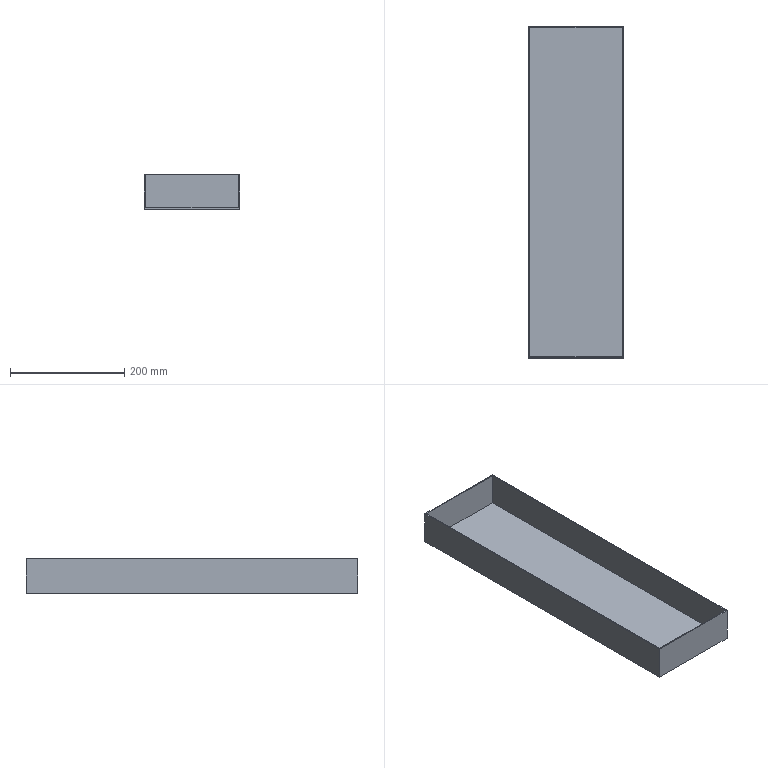Part | NX | features solid 2 | 1 solid | 11 faces | box 167 x 582.059 x 60 mm | volume 367262 mm3 | plane 9 | spline 2
STEP:
#1=CARTESIAN_POINT('',(-360.,302.059,-255.));
#2=VERTEX_POINT('',#1);
#3=CARTESIAN_POINT('',(-360.,-280.,-255.));
#4=VERTEX_POINT('',#3);
#5=CARTESIAN_POINT('',(-360.,-440.,-255.));
#6=DIRECTION('',(0.,1.,0.));
#7=VECTOR('',#6,1000.);
#8=LINE('',#5,#7);
#9=EDGE_CURVE('',#2,#4,#8,.F.);
#10=ORIENTED_EDGE('',*,*,#9,.T.);
#11=CARTESIAN_POINT('',(-360.,-280.,-315.));
#12=VERTEX_POINT('',#11);
#13=CARTESIAN_POINT('',(-360.,-280.,-315.));
#14=DIRECTION('',(0.,0.,1.));
#15=VECTOR('',#14,1000.);
#16=LINE('',#13,#15);
#17=EDGE_CURVE('',#12,#4,#16,.T.);
#18=ORIENTED_EDGE('',*,*,#17,.F.);
#19=CARTESIAN_POINT('',(-360.,302.059,-315.));
#20=VERTEX_POINT('',#19);
#21=CARTESIAN_POINT('',(-360.,-440.,-315.));
#22=DIRECTION('',(0.,1.,0.));
#23=VECTOR('',#22,1000.);
#24=LINE('',#21,#23);
#25=EDGE_CURVE('',#20,#12,#24,.F.);
#26=ORIENTED_EDGE('',*,*,#25,.F.);
#27=CARTESIAN_POINT('',(-360.,302.059,-285.));
#28=DIRECTION('',(0.,0.,1.));
#29=VECTOR('',#28,1000.);
#30=LINE('',#27,#29);
#31=EDGE_CURVE('',#20,#2,#30,.T.);
#32=ORIENTED_EDGE('',*,*,#31,.T.);
#33=EDGE_LOOP('',(#10,#18,#26,#32));
#34=FACE_BOUND('',#33,.T.);
#35=CARTESIAN_POINT('',(-360.,-440.,-315.));
#36=DIRECTION('',(-1.,0.,0.));
#37=DIRECTION('',(0.,0.,1.));
#38=AXIS2_PLACEMENT_3D('',#35,#36,#37);
#39=PLANE('',#38);
#40=ADVANCED_FACE('',(#34),#39,.F.);
#41=CARTESIAN_POINT('',(-527.,-280.,-255.));
#42=VERTEX_POINT('',#41);
#43=CARTESIAN_POINT('',(-780.,-280.,-255.));
#44=DIRECTION('',(-1.,0.,0.));
#45=VECTOR('',#44,1000.);
#46=LINE('',#43,#45);
#47=EDGE_CURVE('',#42,#4,#46,.F.);
#48=ORIENTED_EDGE('',*,*,#47,.F.);
#49=CARTESIAN_POINT('',(-527.,-280.,-315.));
#50=VERTEX_POINT('',#49);
#51=CARTESIAN_POINT('',(-527.,-280.,-315.));
#52=DIRECTION('',(0.,0.,1.));
#53=VECTOR('',#52,1000.);
#54=LINE('',#51,#53);
#55=EDGE_CURVE('',#50,#42,#54,.T.);
#56=ORIENTED_EDGE('',*,*,#55,.F.);
#57=CARTESIAN_POINT('',(-780.,-280.,-315.));
#58=DIRECTION('',(-1.,0.,0.));
#59=VECTOR('',#58,1000.);
#60=LINE('',#57,#59);
#61=EDGE_CURVE('',#50,#12,#60,.F.);
#62=ORIENTED_EDGE('',*,*,#61,.T.);
#63=ORIENTED_EDGE('',*,*,#17,.T.);
#64=EDGE_LOOP('',(#48,#56,#62,#63));
#65=FACE_BOUND('',#64,.T.);
#66=CARTESIAN_POINT('',(-780.,-280.,-315.));
#67=DIRECTION('',(0.,-1.,0.));
#68=DIRECTION('',(0.,0.,-1.));
#69=AXIS2_PLACEMENT_3D('',#66,#67,#68);
#70=PLANE('',#69);
#71=ADVANCED_FACE('',(#65),#70,.T.);
#72=CARTESIAN_POINT('',(-527.,302.059,-255.));
#73=VERTEX_POINT('',#72);
#74=CARTESIAN_POINT('',(-527.,-440.,-255.));
#75=DIRECTION('',(0.,1.,0.));
#76=VECTOR('',#75,1000.);
#77=LINE('',#74,#76);
#78=EDGE_CURVE('',#73,#42,#77,.F.);
#79=ORIENTED_EDGE('',*,*,#78,.F.);
#80=CARTESIAN_POINT('',(-527.,302.059,-315.));
#81=VERTEX_POINT('',#80);
#82=CARTESIAN_POINT('',(-527.,302.059,-315.));
#83=DIRECTION('',(0.,0.,1.));
#84=VECTOR('',#83,1000.);
#85=LINE('',#82,#84);
#86=EDGE_CURVE('',#81,#73,#85,.T.);
#87=ORIENTED_EDGE('',*,*,#86,.F.);
#88=CARTESIAN_POINT('',(-527.,-440.,-315.));
#89=DIRECTION('',(0.,1.,0.));
#90=VECTOR('',#89,1000.);
#91=LINE('',#88,#90);
#92=EDGE_CURVE('',#81,#50,#91,.F.);
#93=ORIENTED_EDGE('',*,*,#92,.T.);
#94=ORIENTED_EDGE('',*,*,#55,.T.);
#95=EDGE_LOOP('',(#79,#87,#93,#94));
#96=FACE_BOUND('',#95,.T.);
#97=CARTESIAN_POINT('',(-527.,-440.,-315.));
#98=DIRECTION('',(-1.,0.,0.));
#99=DIRECTION('',(0.,0.,1.));
#100=AXIS2_PLACEMENT_3D('',#97,#98,#99);
#101=PLANE('',#100);
#102=ADVANCED_FACE('',(#96),#101,.T.);
#103=CARTESIAN_POINT('',(-527.,302.059,-255.));
#104=CARTESIAN_POINT('',(-471.333,302.059,-255.));
#105=CARTESIAN_POINT('',(-415.667,302.059,-255.));
#106=CARTESIAN_POINT('',(-360.,302.059,-255.));
#107=B_SPLINE_CURVE_WITH_KNOTS('',3,(#103,#104,#105,#106),.UNSPECIFIED.,.F.,.F.,(4,4),(-0.037,0.13),.UNSPECIFIED.);
#108=EDGE_CURVE('',#73,#2,#107,.T.);
#109=ORIENTED_EDGE('',*,*,#108,.T.);
#110=ORIENTED_EDGE('',*,*,#31,.F.);
#111=CARTESIAN_POINT('',(-527.,302.059,-315.));
#112=CARTESIAN_POINT('',(-471.333,302.059,-315.));
#113=CARTESIAN_POINT('',(-415.667,302.059,-315.));
#114=CARTESIAN_POINT('',(-360.,302.059,-315.));
#115=B_SPLINE_CURVE_WITH_KNOTS('',3,(#111,#112,#113,#114),.UNSPECIFIED.,.F.,.F.,(4,4),(-0.037,0.13),.UNSPECIFIED.);
#116=EDGE_CURVE('',#81,#20,#115,.T.);
#117=ORIENTED_EDGE('',*,*,#116,.F.);
#118=ORIENTED_EDGE('',*,*,#86,.T.);
#119=EDGE_LOOP('',(#109,#110,#117,#118));
#120=FACE_BOUND('',#119,.T.);
#121=CARTESIAN_POINT('',(-360.,302.059,-315.));
#122=CARTESIAN_POINT('',(-360.,302.059,-255.));
#123=CARTESIAN_POINT('',(-415.667,302.059,-315.));
#124=CARTESIAN_POINT('',(-415.667,302.059,-255.));
#125=CARTESIAN_POINT('',(-471.333,302.059,-315.));
#126=CARTESIAN_POINT('',(-471.333,302.059,-255.));
#127=CARTESIAN_POINT('',(-527.,302.059,-315.));
#128=CARTESIAN_POINT('',(-527.,302.059,-255.));
#129=B_SPLINE_SURFACE_WITH_KNOTS('',3,1,((#121,#122),(#123,#124),(#125,#126),(#127,#128)),.SURF_OF_LINEAR_EXTRUSION.,.F.,.F.,.F.,(4,4),(2,2),(0.3229,0.4727),(0.,1.),.PIECEWISE_BEZIER_KNOTS.);
#130=ADVANCED_FACE('',(#120),#129,.T.);
#131=ORIENTED_EDGE('',*,*,#25,.T.);
#132=ORIENTED_EDGE('',*,*,#61,.F.);
#133=ORIENTED_EDGE('',*,*,#92,.F.);
#134=ORIENTED_EDGE('',*,*,#116,.T.);
#135=EDGE_LOOP('',(#131,#132,#133,#134));
#136=FACE_BOUND('',#135,.T.);
#137=CARTESIAN_POINT('',(-1030.,-440.,-315.));
#138=DIRECTION('',(0.,0.,1.));
#139=DIRECTION('',(0.,1.,0.));
#140=AXIS2_PLACEMENT_3D('',#137,#138,#139);
#141=PLANE('',#140);
#142=ADVANCED_FACE('',(#136),#141,.F.);
#143=CARTESIAN_POINT('',(-525.,300.059,-255.));
#144=VERTEX_POINT('',#143);
#145=CARTESIAN_POINT('',(-362.,300.059,-255.));
#146=VERTEX_POINT('',#145);
#147=CARTESIAN_POINT('',(-525.,300.059,-255.));
#148=CARTESIAN_POINT('',(-470.667,300.059,-255.));
#149=CARTESIAN_POINT('',(-416.333,300.059,-255.));
#150=CARTESIAN_POINT('',(-362.,300.059,-255.));
#151=B_SPLINE_CURVE_WITH_KNOTS('',3,(#147,#148,#149,#150),.UNSPECIFIED.,.F.,.F.,(4,4),(-0.037,0.126),.UNSPECIFIED.);
#152=EDGE_CURVE('',#144,#146,#151,.T.);
#153=ORIENTED_EDGE('',*,*,#152,.T.);
#154=CARTESIAN_POINT('',(-362.,-278.,-255.));
#155=VERTEX_POINT('',#154);
#156=CARTESIAN_POINT('',(-362.,-440.,-255.));
#157=DIRECTION('',(0.,1.,0.));
#158=VECTOR('',#157,1000.);
#159=LINE('',#156,#158);
#160=EDGE_CURVE('',#146,#155,#159,.F.);
#161=ORIENTED_EDGE('',*,*,#160,.T.);
#162=CARTESIAN_POINT('',(-525.,-278.,-255.));
#163=VERTEX_POINT('',#162);
#164=CARTESIAN_POINT('',(-780.,-278.,-255.));
#165=DIRECTION('',(-1.,0.,0.));
#166=VECTOR('',#165,1000.);
#167=LINE('',#164,#166);
#168=EDGE_CURVE('',#163,#155,#167,.F.);
#169=ORIENTED_EDGE('',*,*,#168,.F.);
#170=CARTESIAN_POINT('',(-525.,-440.,-255.));
#171=DIRECTION('',(0.,1.,0.));
#172=VECTOR('',#171,1000.);
#173=LINE('',#170,#172);
#174=EDGE_CURVE('',#144,#163,#173,.F.);
#175=ORIENTED_EDGE('',*,*,#174,.F.);
#176=EDGE_LOOP('',(#153,#161,#169,#175));
#177=FACE_BOUND('',#176,.T.);
#178=ORIENTED_EDGE('',*,*,#9,.F.);
#179=ORIENTED_EDGE('',*,*,#108,.F.);
#180=ORIENTED_EDGE('',*,*,#78,.T.);
#181=ORIENTED_EDGE('',*,*,#47,.T.);
#182=EDGE_LOOP('',(#178,#179,#180,#181));
#183=FACE_BOUND('',#182,.T.);
#184=CARTESIAN_POINT('',(-1030.,-440.,-255.));
#185=DIRECTION('',(0.,0.,1.));
#186=DIRECTION('',(0.,1.,0.));
#187=AXIS2_PLACEMENT_3D('',#184,#185,#186);
#188=PLANE('',#187);
#189=ADVANCED_FACE('',(#177,#183),#188,.T.);
#190=ORIENTED_EDGE('',*,*,#160,.F.);
#191=CARTESIAN_POINT('',(-362.,300.059,-313.));
#192=VERTEX_POINT('',#191);
#193=CARTESIAN_POINT('',(-362.,300.059,-313.));
#194=DIRECTION('',(0.,0.,1.));
#195=VECTOR('',#194,1000.);
#196=LINE('',#193,#195);
#197=EDGE_CURVE('',#192,#146,#196,.T.);
#198=ORIENTED_EDGE('',*,*,#197,.F.);
#199=CARTESIAN_POINT('',(-362.,-278.,-313.));
#200=VERTEX_POINT('',#199);
#201=CARTESIAN_POINT('',(-362.,-440.,-313.));
#202=DIRECTION('',(0.,1.,0.));
#203=VECTOR('',#202,1000.);
#204=LINE('',#201,#203);
#205=EDGE_CURVE('',#192,#200,#204,.F.);
#206=ORIENTED_EDGE('',*,*,#205,.T.);
#207=CARTESIAN_POINT('',(-362.,-278.,-315.));
#208=DIRECTION('',(0.,0.,1.));
#209=VECTOR('',#208,1000.);
#210=LINE('',#207,#209);
#211=EDGE_CURVE('',#200,#155,#210,.T.);
#212=ORIENTED_EDGE('',*,*,#211,.T.);
#213=EDGE_LOOP('',(#190,#198,#206,#212));
#214=FACE_BOUND('',#213,.T.);
#215=CARTESIAN_POINT('',(-362.,-440.,-315.));
#216=DIRECTION('',(-1.,0.,0.));
#217=DIRECTION('',(0.,0.,1.));
#218=AXIS2_PLACEMENT_3D('',#215,#216,#217);
#219=PLANE('',#218);
#220=ADVANCED_FACE('',(#214),#219,.T.);
#221=ORIENTED_EDGE('',*,*,#168,.T.);
#222=ORIENTED_EDGE('',*,*,#211,.F.);
#223=CARTESIAN_POINT('',(-525.,-278.,-313.));
#224=VERTEX_POINT('',#223);
#225=CARTESIAN_POINT('',(-780.,-278.,-313.));
#226=DIRECTION('',(-1.,0.,0.));
#227=VECTOR('',#226,1000.);
#228=LINE('',#225,#227);
#229=EDGE_CURVE('',#224,#200,#228,.F.);
#230=ORIENTED_EDGE('',*,*,#229,.F.);
#231=CARTESIAN_POINT('',(-525.,-278.,-315.));
#232=DIRECTION('',(0.,0.,1.));
#233=VECTOR('',#232,1000.);
#234=LINE('',#231,#233);
#235=EDGE_CURVE('',#224,#163,#234,.T.);
#236=ORIENTED_EDGE('',*,*,#235,.T.);
#237=EDGE_LOOP('',(#221,#222,#230,#236));
#238=FACE_BOUND('',#237,.T.);
#239=CARTESIAN_POINT('',(-780.,-278.,-315.));
#240=DIRECTION('',(0.,-1.,0.));
#241=DIRECTION('',(0.,0.,-1.));
#242=AXIS2_PLACEMENT_3D('',#239,#240,#241);
#243=PLANE('',#242);
#244=ADVANCED_FACE('',(#238),#243,.F.);
#245=ORIENTED_EDGE('',*,*,#174,.T.);
#246=ORIENTED_EDGE('',*,*,#235,.F.);
#247=CARTESIAN_POINT('',(-525.,300.059,-313.));
#248=VERTEX_POINT('',#247);
#249=CARTESIAN_POINT('',(-525.,-440.,-313.));
#250=DIRECTION('',(0.,1.,0.));
#251=VECTOR('',#250,1000.);
#252=LINE('',#249,#251);
#253=EDGE_CURVE('',#248,#224,#252,.F.);
#254=ORIENTED_EDGE('',*,*,#253,.F.);
#255=CARTESIAN_POINT('',(-525.,300.059,-284.));
#256=DIRECTION('',(0.,0.,1.));
#257=VECTOR('',#256,1000.);
#258=LINE('',#255,#257);
#259=EDGE_CURVE('',#248,#144,#258,.T.);
#260=ORIENTED_EDGE('',*,*,#259,.T.);
#261=EDGE_LOOP('',(#245,#246,#254,#260));
#262=FACE_BOUND('',#261,.T.);
#263=CARTESIAN_POINT('',(-525.,-440.,-315.));
#264=DIRECTION('',(-1.,0.,0.));
#265=DIRECTION('',(0.,0.,1.));
#266=AXIS2_PLACEMENT_3D('',#263,#264,#265);
#267=PLANE('',#266);
#268=ADVANCED_FACE('',(#262),#267,.F.);
#269=ORIENTED_EDGE('',*,*,#152,.F.);
#270=ORIENTED_EDGE('',*,*,#259,.F.);
#271=CARTESIAN_POINT('',(-525.,300.059,-313.));
#272=CARTESIAN_POINT('',(-470.667,300.059,-313.));
#273=CARTESIAN_POINT('',(-416.333,300.059,-313.));
#274=CARTESIAN_POINT('',(-362.,300.059,-313.));
#275=B_SPLINE_CURVE_WITH_KNOTS('',3,(#271,#272,#273,#274),.UNSPECIFIED.,.F.,.F.,(4,4),(-0.037,0.126),.UNSPECIFIED.);
#276=EDGE_CURVE('',#248,#192,#275,.T.);
#277=ORIENTED_EDGE('',*,*,#276,.T.);
#278=ORIENTED_EDGE('',*,*,#197,.T.);
#279=EDGE_LOOP('',(#269,#270,#277,#278));
#280=FACE_BOUND('',#279,.T.);
#281=CARTESIAN_POINT('',(-362.,300.059,-313.));
#282=CARTESIAN_POINT('',(-362.,300.059,-255.));
#283=CARTESIAN_POINT('',(-416.333,300.059,-313.));
#284=CARTESIAN_POINT('',(-416.333,300.059,-255.));
#285=CARTESIAN_POINT('',(-470.667,300.059,-313.));
#286=CARTESIAN_POINT('',(-470.667,300.059,-255.));
#287=CARTESIAN_POINT('',(-525.,300.059,-313.));
#288=CARTESIAN_POINT('',(-525.,300.059,-255.));
#289=B_SPLINE_SURFACE_WITH_KNOTS('',3,1,((#281,#282),(#283,#284),(#285,#286),(#287,#288)),.SURF_OF_LINEAR_EXTRUSION.,.F.,.F.,.F.,(4,4),(2,2),(0.,1.),(0.,1.),.PIECEWISE_BEZIER_KNOTS.);
#290=ADVANCED_FACE('',(#280),#289,.F.);
#291=ORIENTED_EDGE('',*,*,#205,.F.);
#292=ORIENTED_EDGE('',*,*,#276,.F.);
#293=ORIENTED_EDGE('',*,*,#253,.T.);
#294=ORIENTED_EDGE('',*,*,#229,.T.);
#295=EDGE_LOOP('',(#291,#292,#293,#294));
#296=FACE_BOUND('',#295,.T.);
#297=CARTESIAN_POINT('',(-1030.,-440.,-313.));
#298=DIRECTION('',(0.,0.,1.));
#299=DIRECTION('',(0.,1.,0.));
#300=AXIS2_PLACEMENT_3D('',#297,#298,#299);
#301=PLANE('',#300);
#302=ADVANCED_FACE('',(#296),#301,.T.);
#303=CLOSED_SHELL('',(#40,#71,#102,#130,#142,#189,#220,#244,#268,#290,#302));
#304=MANIFOLD_SOLID_BREP('',#303);
#305=(LENGTH_UNIT()NAMED_UNIT(*)SI_UNIT(.MILLI.,.METRE.));
#306=UNCERTAINTY_MEASURE_WITH_UNIT(LENGTH_MEASURE(0.0508),#305,'','');
#307=(NAMED_UNIT(*)PLANE_ANGLE_UNIT()SI_UNIT($,.RADIAN.));
#308=(NAMED_UNIT(*)SI_UNIT($,.STERADIAN.)SOLID_ANGLE_UNIT());
#309=(GEOMETRIC_REPRESENTATION_CONTEXT(3)GLOBAL_UNCERTAINTY_ASSIGNED_CONTEXT((#306))GLOBAL_UNIT_ASSIGNED_CONTEXT((#305,#307,#308))REPRESENTATION_CONTEXT('',''));
#310=ADVANCED_BREP_SHAPE_REPRESENTATION('',(#304),#309);